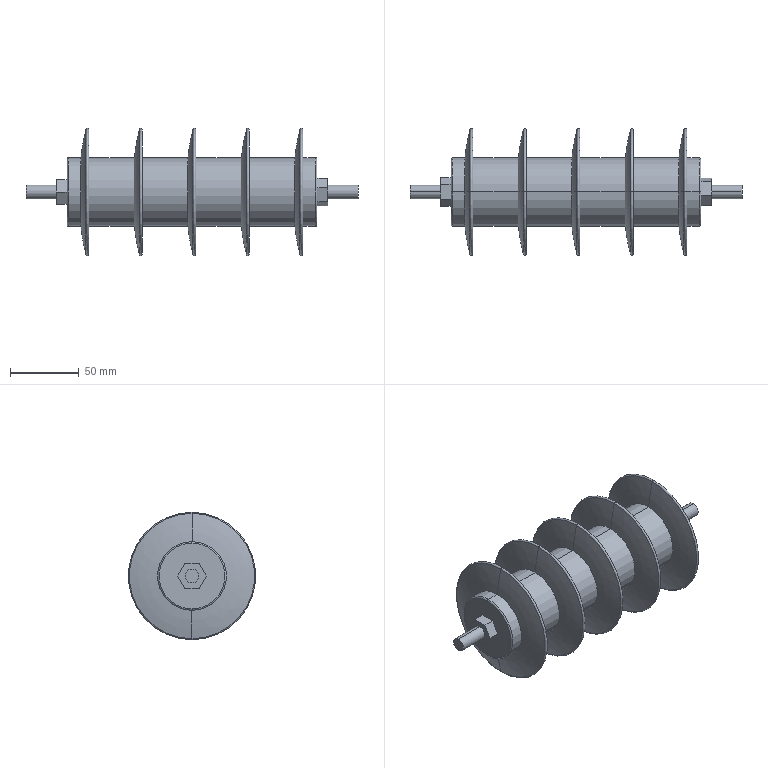Part | STEP file | Surge arrester | 1 solid | 63 faces | box 242 x 92.835 x 92.835 mm | volume 456691 mm3 | plane 23 | cylinder 16 | torus 14 | other 10 | commonest cylinder face diameters 50 x12 10 x4